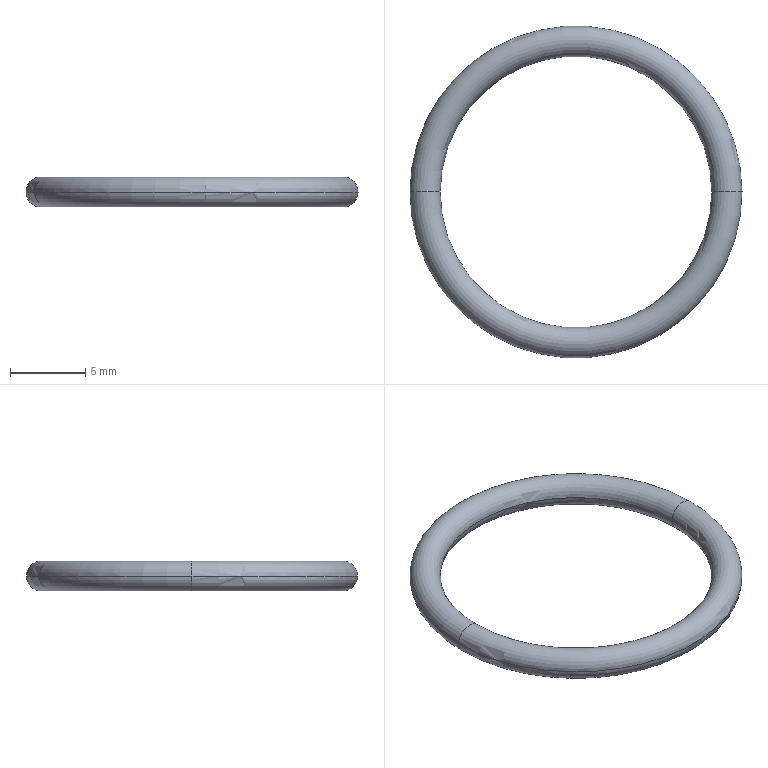Part | SolidWorks | features RefAxis 1, Revolution 1 | 1 solid | 4 faces | box 22 x 22 x 2 mm | volume 197.392 mm3 | torus 4
STEP:
#1=CARTESIAN_POINT('',(11.,0.,0.));
#2=VERTEX_POINT('',#1);
#3=CARTESIAN_POINT('',(9.,0.,0.));
#4=VERTEX_POINT('',#3);
#5=CARTESIAN_POINT('',(10.,0.,0.));
#6=DIRECTION('',(0.,1.,0.));
#7=DIRECTION('',(-1.,0.,0.));
#8=AXIS2_PLACEMENT_3D('',#5,#6,#7);
#9=CIRCLE('',#8,1.);
#10=EDGE_CURVE('',#2,#4,#9,.T.);
#11=ORIENTED_EDGE('',*,*,#10,.F.);
#12=CARTESIAN_POINT('',(-11.,0.,0.));
#13=VERTEX_POINT('',#12);
#14=CARTESIAN_POINT('',(0.,0.,0.));
#15=DIRECTION('',(0.,0.,-1.));
#16=DIRECTION('',(-1.,0.,0.));
#17=AXIS2_PLACEMENT_3D('',#14,#15,#16);
#18=CIRCLE('',#17,11.);
#19=EDGE_CURVE('',#2,#13,#18,.T.);
#20=ORIENTED_EDGE('',*,*,#19,.T.);
#21=CARTESIAN_POINT('',(-9.,0.,0.));
#22=VERTEX_POINT('',#21);
#23=CARTESIAN_POINT('',(-10.,0.,0.));
#24=DIRECTION('',(0.,-1.,0.));
#25=DIRECTION('',(0.,0.,-1.));
#26=AXIS2_PLACEMENT_3D('',#23,#24,#25);
#27=CIRCLE('',#26,1.);
#28=EDGE_CURVE('',#13,#22,#27,.T.);
#29=ORIENTED_EDGE('',*,*,#28,.T.);
#30=CARTESIAN_POINT('',(0.,0.,0.));
#31=DIRECTION('',(0.,0.,-1.));
#32=DIRECTION('',(-1.,0.,0.));
#33=AXIS2_PLACEMENT_3D('',#30,#31,#32);
#34=CIRCLE('',#33,9.);
#35=EDGE_CURVE('',#4,#22,#34,.T.);
#36=ORIENTED_EDGE('',*,*,#35,.F.);
#37=EDGE_LOOP('',(#11,#20,#29,#36));
#38=FACE_OUTER_BOUND('',#37,.T.);
#39=CARTESIAN_POINT('',(0.,0.,0.));
#40=DIRECTION('',(0.,0.,-1.));
#41=DIRECTION('',(-1.,0.,0.));
#42=AXIS2_PLACEMENT_3D('',#39,#40,#41);
#43=TOROIDAL_SURFACE('',#42,10.,1.);
#44=ADVANCED_FACE('',(#38),#43,.T.);
#45=ORIENTED_EDGE('',*,*,#28,.F.);
#46=CARTESIAN_POINT('',(0.,0.,0.));
#47=DIRECTION('',(0.,0.,-1.));
#48=DIRECTION('',(-1.,0.,0.));
#49=AXIS2_PLACEMENT_3D('',#46,#47,#48);
#50=CIRCLE('',#49,11.);
#51=EDGE_CURVE('',#13,#2,#50,.T.);
#52=ORIENTED_EDGE('',*,*,#51,.T.);
#53=ORIENTED_EDGE('',*,*,#10,.T.);
#54=CARTESIAN_POINT('',(0.,0.,0.));
#55=DIRECTION('',(0.,0.,-1.));
#56=DIRECTION('',(-1.,0.,0.));
#57=AXIS2_PLACEMENT_3D('',#54,#55,#56);
#58=CIRCLE('',#57,9.);
#59=EDGE_CURVE('',#22,#4,#58,.T.);
#60=ORIENTED_EDGE('',*,*,#59,.F.);
#61=EDGE_LOOP('',(#45,#52,#53,#60));
#62=FACE_OUTER_BOUND('',#61,.T.);
#63=CARTESIAN_POINT('',(0.,0.,0.));
#64=DIRECTION('',(0.,0.,-1.));
#65=DIRECTION('',(-1.,0.,0.));
#66=AXIS2_PLACEMENT_3D('',#63,#64,#65);
#67=TOROIDAL_SURFACE('',#66,10.,1.);
#68=ADVANCED_FACE('',(#62),#67,.T.);
#69=ORIENTED_EDGE('',*,*,#51,.F.);
#70=CARTESIAN_POINT('',(-10.,0.,0.));
#71=DIRECTION('',(0.,-1.,0.));
#72=DIRECTION('',(0.,0.,-1.));
#73=AXIS2_PLACEMENT_3D('',#70,#71,#72);
#74=CIRCLE('',#73,1.);
#75=EDGE_CURVE('',#22,#13,#74,.T.);
#76=ORIENTED_EDGE('',*,*,#75,.F.);
#77=ORIENTED_EDGE('',*,*,#59,.T.);
#78=CARTESIAN_POINT('',(10.,0.,0.));
#79=DIRECTION('',(0.,1.,0.));
#80=DIRECTION('',(-1.,0.,0.));
#81=AXIS2_PLACEMENT_3D('',#78,#79,#80);
#82=CIRCLE('',#81,1.);
#83=EDGE_CURVE('',#4,#2,#82,.T.);
#84=ORIENTED_EDGE('',*,*,#83,.T.);
#85=EDGE_LOOP('',(#69,#76,#77,#84));
#86=FACE_OUTER_BOUND('',#85,.T.);
#87=CARTESIAN_POINT('',(0.,0.,0.));
#88=DIRECTION('',(0.,0.,-1.));
#89=DIRECTION('',(-1.,0.,0.));
#90=AXIS2_PLACEMENT_3D('',#87,#88,#89);
#91=TOROIDAL_SURFACE('',#90,10.,1.);
#92=ADVANCED_FACE('',(#86),#91,.T.);
#93=ORIENTED_EDGE('',*,*,#19,.F.);
#94=ORIENTED_EDGE('',*,*,#83,.F.);
#95=ORIENTED_EDGE('',*,*,#35,.T.);
#96=ORIENTED_EDGE('',*,*,#75,.T.);
#97=EDGE_LOOP('',(#93,#94,#95,#96));
#98=FACE_OUTER_BOUND('',#97,.T.);
#99=CARTESIAN_POINT('',(0.,0.,0.));
#100=DIRECTION('',(0.,0.,-1.));
#101=DIRECTION('',(-1.,0.,0.));
#102=AXIS2_PLACEMENT_3D('',#99,#100,#101);
#103=TOROIDAL_SURFACE('',#102,10.,1.);
#104=ADVANCED_FACE('',(#98),#103,.T.);
#105=CLOSED_SHELL('',(#44,#68,#92,#104));
#106=MANIFOLD_SOLID_BREP('',#105);
#107=CARTESIAN_POINT('',(0.,0.,0.));
#108=DIRECTION('',(0.,0.,1.));
#109=DIRECTION('',(1.,0.,0.));
#110=AXIS2_PLACEMENT_3D('',#107,#108,#109);
#111=(LENGTH_UNIT()NAMED_UNIT(*)SI_UNIT(.MILLI.,.METRE.));
#112=UNCERTAINTY_MEASURE_WITH_UNIT(LENGTH_MEASURE(0.00001),#111,'','');
#113=(NAMED_UNIT(*)PLANE_ANGLE_UNIT()SI_UNIT($,.RADIAN.));
#114=(NAMED_UNIT(*)SI_UNIT($,.STERADIAN.)SOLID_ANGLE_UNIT());
#115=(GEOMETRIC_REPRESENTATION_CONTEXT(3)GLOBAL_UNCERTAINTY_ASSIGNED_CONTEXT((#112))GLOBAL_UNIT_ASSIGNED_CONTEXT((#111,#113,#114))REPRESENTATION_CONTEXT('',''));
#116=ADVANCED_BREP_SHAPE_REPRESENTATION('',(#106,#110),#115);